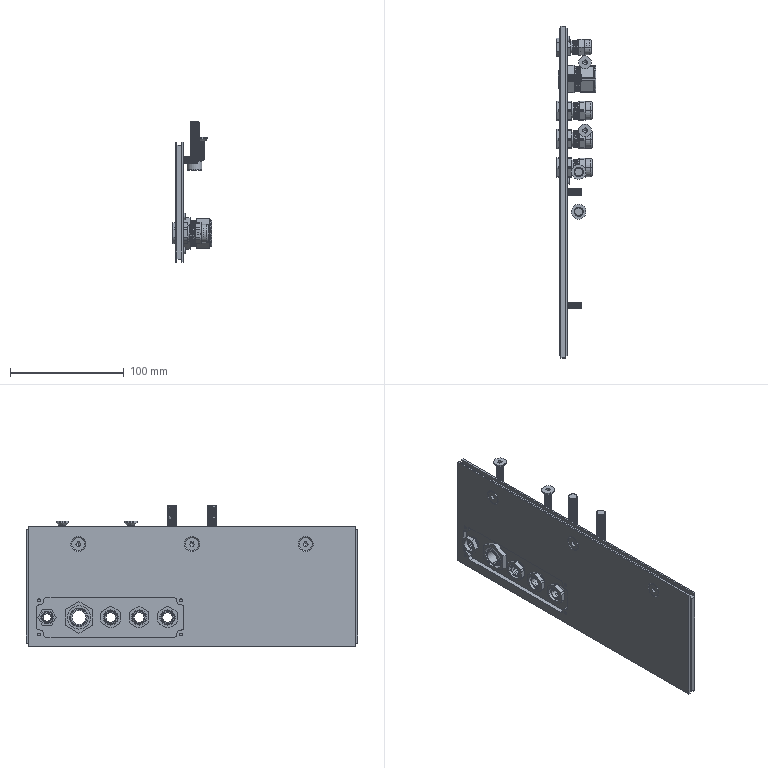Part | SolidWorks | 24 solids | 3095 faces | volume 207636 mm3 | cone 1324 | cylinder 1127 | plane 582 | spline 40 | torus 14 | sphere 8 | commonest cylinder face diameters 6 x288 8 x177 3 x144 11 x115 18.5 x63 13.5 x48